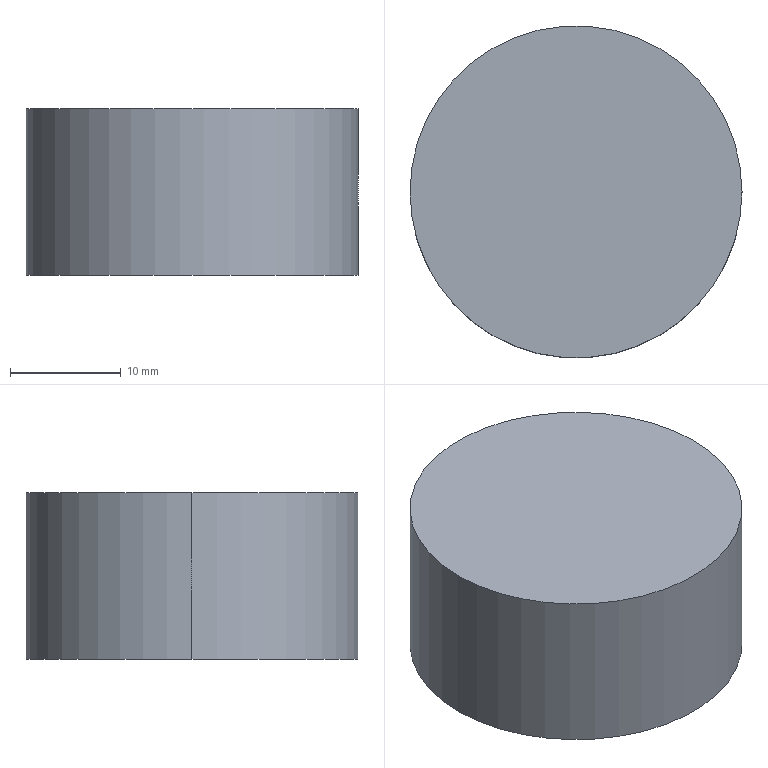Part | SolidWorks | features Extrusion 1 | 1 solid | 4 faces | box 30 x 30 x 15 mm | volume 10603 mm3 | cylinder 2 | plane 2 | commonest cylinder face diameters 30 x2
STEP:
#1=CARTESIAN_POINT('',(67.709,73.328,15.));
#2=VERTEX_POINT('',#1);
#3=CARTESIAN_POINT('',(37.709,73.328,15.));
#4=VERTEX_POINT('',#3);
#5=CARTESIAN_POINT('',(52.709,73.328,15.));
#6=DIRECTION('',(0.,0.,1.));
#7=DIRECTION('',(1.,0.,0.));
#8=AXIS2_PLACEMENT_3D('',#5,#6,#7);
#9=CIRCLE('',#8,15.);
#10=EDGE_CURVE('',#2,#4,#9,.T.);
#11=ORIENTED_EDGE('',*,*,#10,.F.);
#12=CARTESIAN_POINT('',(67.709,73.328,0.));
#13=VERTEX_POINT('',#12);
#14=CARTESIAN_POINT('',(67.709,73.328,15.));
#15=DIRECTION('',(0.,0.,-1.));
#16=VECTOR('',#15,1000.);
#17=LINE('',#14,#16);
#18=EDGE_CURVE('',#2,#13,#17,.T.);
#19=ORIENTED_EDGE('',*,*,#18,.T.);
#20=CARTESIAN_POINT('',(37.709,73.328,0.));
#21=VERTEX_POINT('',#20);
#22=CARTESIAN_POINT('',(52.709,73.328,0.));
#23=DIRECTION('',(0.,0.,1.));
#24=DIRECTION('',(1.,0.,0.));
#25=AXIS2_PLACEMENT_3D('',#22,#23,#24);
#26=CIRCLE('',#25,15.);
#27=EDGE_CURVE('',#13,#21,#26,.T.);
#28=ORIENTED_EDGE('',*,*,#27,.T.);
#29=CARTESIAN_POINT('',(37.709,73.328,15.));
#30=DIRECTION('',(0.,0.,-1.));
#31=VECTOR('',#30,1000.);
#32=LINE('',#29,#31);
#33=EDGE_CURVE('',#4,#21,#32,.T.);
#34=ORIENTED_EDGE('',*,*,#33,.F.);
#35=EDGE_LOOP('',(#11,#19,#28,#34));
#36=FACE_OUTER_BOUND('',#35,.T.);
#37=CARTESIAN_POINT('',(52.709,73.328,15.));
#38=DIRECTION('',(0.,0.,-1.));
#39=DIRECTION('',(-1.,0.,0.));
#40=AXIS2_PLACEMENT_3D('',#37,#38,#39);
#41=CYLINDRICAL_SURFACE('',#40,15.);
#42=ADVANCED_FACE('',(#36),#41,.T.);
#43=ORIENTED_EDGE('',*,*,#18,.F.);
#44=CARTESIAN_POINT('',(52.709,73.328,15.));
#45=DIRECTION('',(0.,0.,1.));
#46=DIRECTION('',(1.,0.,0.));
#47=AXIS2_PLACEMENT_3D('',#44,#45,#46);
#48=CIRCLE('',#47,15.);
#49=EDGE_CURVE('',#4,#2,#48,.T.);
#50=ORIENTED_EDGE('',*,*,#49,.F.);
#51=ORIENTED_EDGE('',*,*,#33,.T.);
#52=CARTESIAN_POINT('',(52.709,73.328,0.));
#53=DIRECTION('',(0.,0.,1.));
#54=DIRECTION('',(1.,0.,0.));
#55=AXIS2_PLACEMENT_3D('',#52,#53,#54);
#56=CIRCLE('',#55,15.);
#57=EDGE_CURVE('',#21,#13,#56,.T.);
#58=ORIENTED_EDGE('',*,*,#57,.T.);
#59=EDGE_LOOP('',(#43,#50,#51,#58));
#60=FACE_OUTER_BOUND('',#59,.T.);
#61=CARTESIAN_POINT('',(52.709,73.328,15.));
#62=DIRECTION('',(0.,0.,-1.));
#63=DIRECTION('',(-1.,0.,0.));
#64=AXIS2_PLACEMENT_3D('',#61,#62,#63);
#65=CYLINDRICAL_SURFACE('',#64,15.);
#66=ADVANCED_FACE('',(#60),#65,.T.);
#67=ORIENTED_EDGE('',*,*,#49,.T.);
#68=ORIENTED_EDGE('',*,*,#10,.T.);
#69=EDGE_LOOP('',(#67,#68));
#70=FACE_OUTER_BOUND('',#69,.T.);
#71=CARTESIAN_POINT('',(52.709,73.328,15.));
#72=DIRECTION('',(0.,0.,1.));
#73=DIRECTION('',(1.,0.,0.));
#74=AXIS2_PLACEMENT_3D('',#71,#72,#73);
#75=PLANE('',#74);
#76=ADVANCED_FACE('',(#70),#75,.T.);
#77=ORIENTED_EDGE('',*,*,#57,.F.);
#78=ORIENTED_EDGE('',*,*,#27,.F.);
#79=EDGE_LOOP('',(#77,#78));
#80=FACE_OUTER_BOUND('',#79,.T.);
#81=CARTESIAN_POINT('',(52.709,73.328,0.));
#82=DIRECTION('',(0.,0.,1.));
#83=DIRECTION('',(1.,0.,0.));
#84=AXIS2_PLACEMENT_3D('',#81,#82,#83);
#85=PLANE('',#84);
#86=ADVANCED_FACE('',(#80),#85,.F.);
#87=CLOSED_SHELL('',(#42,#66,#76,#86));
#88=MANIFOLD_SOLID_BREP('',#87);
#89=CARTESIAN_POINT('',(0.,0.,0.));
#90=DIRECTION('',(0.,0.,1.));
#91=DIRECTION('',(1.,0.,0.));
#92=AXIS2_PLACEMENT_3D('',#89,#90,#91);
#93=(LENGTH_UNIT()NAMED_UNIT(*)SI_UNIT(.MILLI.,.METRE.));
#94=UNCERTAINTY_MEASURE_WITH_UNIT(LENGTH_MEASURE(0.00001),#93,'','');
#95=(NAMED_UNIT(*)PLANE_ANGLE_UNIT()SI_UNIT($,.RADIAN.));
#96=(NAMED_UNIT(*)SI_UNIT($,.STERADIAN.)SOLID_ANGLE_UNIT());
#97=(GEOMETRIC_REPRESENTATION_CONTEXT(3)GLOBAL_UNCERTAINTY_ASSIGNED_CONTEXT((#94))GLOBAL_UNIT_ASSIGNED_CONTEXT((#93,#95,#96))REPRESENTATION_CONTEXT('',''));
#98=ADVANCED_BREP_SHAPE_REPRESENTATION('',(#88,#92),#97);